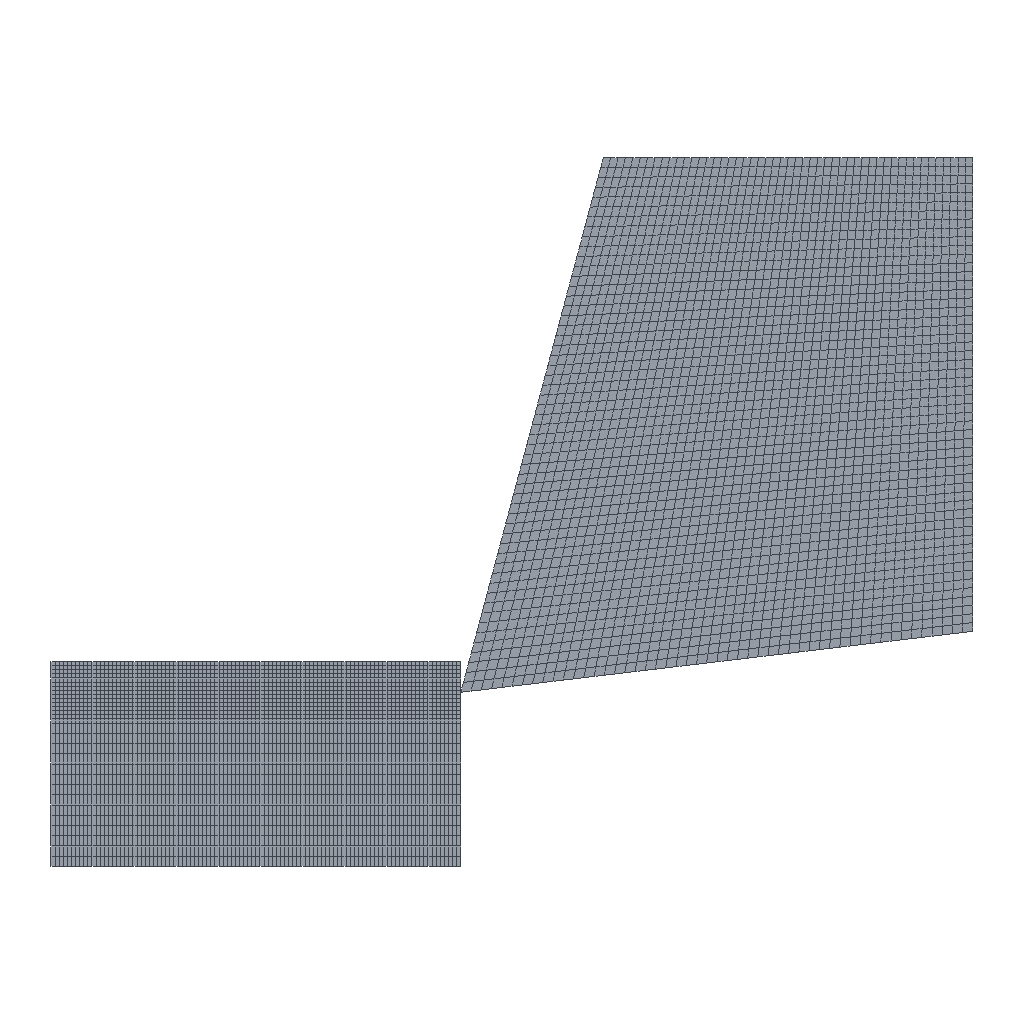Simulation study | abaqus
Set-up summary:
category,name,step,type,value,unit,region
solver,abaqus,,Abaqus/CAE 2024
units,mm-N-s-tonne (MPa),,inferred,E=960000 density=3.5e-09
analysis,Step-1,,dynamic temp-displacement,nlgeom=True; time_period=0.002
mesh,nodes,,,5836
mesh,elements,,,5600
element_type,CPE4RT,,,5600
material,DOMAND,,E,960000
material,DOMAND,,nu,0.2
material,DOMAND,,density,3.5e-09
material,DOMAND,,conductivity,1674.72
material,DOMAND,,specific_heat,5.16e+08
material,DOMAND,,cte,1.18e-06
material,DOMAND,,behaviors,conductivity; expansion; specific heat
material,TC4,,E,105000
material,TC4,,nu,0.33
material,TC4,,density,4.43e-09
material,TC4,,conductivity,5.44
material,TC4,,cte,9e-06
material,TC4,,behaviors,conductivity; damage initiation; damage evolution; expansion
section,TC4,,solid section,,,_PickedSet2
section,DOMAND,,solid section,,,_PickedSet2
load,Predefined,initial,initial condition temperature
bc,BC-1,initial,encastre,[dofs=ENCASTRE],,_PickedSet10
bc,BC-2,Step-1,velocity,"-1000 [dofs=rz,x,y n=3]",,_PickedSet11
contact,Int-1,Step-1,contact pair,interaction=INTPROP-1; friction=0.2; behavior=hard,,tool-1.Surf-tool / TC4-1_Set-all_CNS_
contact,Int-2,Step-1,general contact,interaction=IntProp-2
constraint,rigid body,,,1
Abaqus input file, long lists of numbers shortened:
*Heading
** Job name: deck Model name: Model-2-Copy
** Generated by: Abaqus/CAE 2024
*Preprint, echo=NO, model=NO, history=NO, contact=NO
**
** PARTS
**
*Part, name=TC4
*Node
      1,           2., -0.3
      2,           0., -0.3
** (3028 more lines like these left out)
*Element, type=CPE4RT
   1,    1,    7,  358,  230
   2,    7,    8,  359,  358
** (2898 more lines like these left out)
*Nset, nset=_PickedSet2, internal, generate
    1,  3030,     1
*Elset, elset=_PickedSet2, internal, generate
    1,  2900,     1
*Nset, nset=Set-all
    1,    2,    5,    6,    7,    8,    9,   10,   11,   12,   13,   14,   15,   16,   17,   18
   19,   20,   21,   22,   23,   24,   25,   26,   27,   28,   29,   30,   31,   32,   33,   34
** (99 more lines like these left out)
** Section: TC4
*Solid Section, elset=_PickedSet2, material=TC4
,
*End Part
**
*Part, name=tool
*Node
      1,           0.,           0.
      2, 0.05, 0.005956
** (2803 more lines like these left out)
*Element, type=CPE4RT
   1,    1,    2,   53,   52
   2,    2,    3,   54,   53
** (2698 more lines like these left out)
*Node
   2806,          2.5,   2.61,           0.
*Nset, nset=tool-RefPt_, internal
2806,
*Nset, nset=_PickedSet2, internal, generate
    1,  2805,     1
*Elset, elset=_PickedSet2, internal, generate
    1,  2700,     1
*Elset, elset=_Surf-tool_S1, internal, generate
  1,  50,   1
*Elset, elset=_Surf-tool_S4, internal, generate
    1,  2651,    50
*Surface, type=ELEMENT, name=Surf-tool
_Surf-tool_S1, S1
_Surf-tool_S4, S4
** Section: Tool
*Solid Section, elset=_PickedSet2, material=DOMAND
,
*End Part
**
**
** ASSEMBLY
**
*Assembly, name=Assembly
**
*Instance, name=TC4-1, part=TC4
*End Instance
**
*Instance, name=tool-1, part=tool
          2.,        -0.15,           0.
*End Instance
**
*Nset, nset=Set-RP, instance=tool-1
 2806,
*Nset, nset=_PickedSet6, internal, instance=tool-1
 2806,
*Nset, nset=_PickedSet7, internal, instance=tool-1, generate
    1,  2805,     1
*Elset, elset=_PickedSet7, internal, instance=tool-1, generate
    1,  2700,     1
*Nset, nset=_PickedSet9, internal, instance=tool-1
 2806,
*Nset, nset=_PickedSet10, internal, instance=TC4-1
   1,   2,   3,   4,   6, 106, 107, 108, 109, 110, 111, 112, 113, 114, 115, 116
 117, 118, 119, 120, 121, 122, 123, 124, 125, 126, 127, 128, 129, 130, 131, 132
** (7 more lines like these left out)
*Elset, elset=_PickedSet10, internal, instance=TC4-1
    1,  100,  101,  200,  201,  300,  301,  400,  401,  500,  501,  600,  601,  700,  701,  800
  801,  900,  901, 1000, 1001, 1100, 1101, 1200, 1201, 1300, 1301, 1302, 1303, 1304, 1305, 1306
** (7 more lines like these left out)
*Nset, nset=_PickedSet11, internal, instance=tool-1
 2806,
*Nset, nset=_PickedSet12, internal, instance=TC4-1, generate
    1,  3030,     1
*Nset, nset=_PickedSet12, internal, instance=tool-1, generate
    1,  2805,     1
*Elset, elset=_PickedSet12, internal, instance=TC4-1, generate
    1,  2900,     1
*Elset, elset=_PickedSet12, internal, instance=tool-1, generate
    1,  2700,     1
*Elset, elset=__PickedSurf8_S1, internal, instance=tool-1, generate
  1,  50,   1
*Elset, elset=__PickedSurf8_S2, internal, instance=tool-1, generate
   50,  2700,    50
*Elset, elset=__PickedSurf8_S4, internal, instance=tool-1, generate
    1,  2651,    50
*Surface, type=ELEMENT, name=_PickedSurf8, internal
__PickedSurf8_S1, S1
__PickedSurf8_S2, S2
__PickedSurf8_S4, S4
*Surface, type=NODE, name=TC4-1_Set-all_CNS_, internal
TC4-1.Set-all, 1.
** Constraint: Constraint-2
*Rigid Body, ref node=_PickedSet6, elset=_PickedSet7
*End Assembly
**
** MATERIALS
**
*Material, name=DOMAND
*Conductivity
 1674.72,
*Density
 3.5e-09,
*Elastic
960000., 0.2
*Expansion
 1.18e-06,
*Specific Heat
 5.16e+08,
*Material, name=TC4
*Conductivity
  5.44, 20.
   6.7,100.
  8.79,200.
 10.47,300.
 12.56,400.
 14.24,500.
 15.49,600.
*Damage Initiation, criterion=JOHNSON COOK
 -0.09,  0.25,  -0.5, 0.014,  3.87, 1650.,   20.,    1.
*Damage Evolution, type=DISPLACEMENT
 0.02,
*Density
 4.43e-09,
*Elastic
105000., 0.33
*Expansion
 9e-06,20.
*Inelastic Heat Fraction
        0.95,
*Plastic, hardening=JOHNSON COOK
875., 793., 0.38, 0.71,1650.,  20.
*Rate Dependent, type=JOHNSON COOK
 0.01,1.
*Specific Heat
 6.78e+08,100.
 6.91e+08,200.
 7.03e+08,300.
 7.41e+08,400.
 7.54e+08,500.
 8.79e+08,600.
**
** INTERACTION PROPERTIES
**
*Surface Interaction, name=INTPROP-1
*Friction
 0.2,
*Surface Behavior, pressure-overclosure=HARD
*Surface Interaction, name=IntProp-2
**
** BOUNDARY CONDITIONS
**
** Name: BC-1 Type: Symmetry/Antisymmetry/Encastre
*Boundary
_PickedSet10, ENCASTRE
**
** PREDEFINED FIELDS
**
** Name: Predefined Field-1   Type: Temperature
*Initial Conditions, type=TEMPERATURE
_PickedSet12, 25.
** ----------------------------------------------------------------
**
** STEP: Step-1
**
*Step, name=Step-1, nlgeom=YES
*Dynamic Temperature-displacement, Explicit
, 0.002
*Bulk Viscosity
0.06, 1.2
** Mass Scaling: Semi-Automatic
**               Whole Model
*Fixed Mass Scaling, factor=1000.
**
** BOUNDARY CONDITIONS
**
** Name: BC-2 Type: Velocity/Angular velocity
*Boundary, type=VELOCITY
_PickedSet11, 1, 1, -1000.
_PickedSet11, 2, 2
_PickedSet11, 6, 6
**
** INTERACTIONS
**
** Interaction: Int-1
*Contact Pair, interaction=INTPROP-1, mechanical constraint=PENALTY, cpset=Int-1
tool-1.Surf-tool, TC4-1_Set-all_CNS_
** Interaction: Int-2
*Contact, op=NEW
*Contact Inclusions, ALL EXTERIOR
*Contact Property Assignment
 ,  , IntProp-2
**
** OUTPUT REQUESTS
**
*Restart, write, number interval=1, time marks=NO
**
** FIELD OUTPUT: F-Output-1
**
*Output, field, number interval=500
*Node Output
NT, RF
*Element Output, directions=YES
CFAILURE, DAMAGESHR, DMICRT, E, EVF, S, SDEG, STATUS, TEMP
*Contact Output
CSDMG, CSTRESS
*Output, history, frequency=0
*End Step
Results summary:
result,odb.job_status,,,JOB_STATUS_UNKNOWN,"consistent, unstated (Abaqus has no unit system)"
result,steps[0].procedure,Step-1,,"*DYNAMIC TEMPERATURE-DISPLACEMENT, EXPLICT","consistent, unstated (Abaqus has no unit system)"
result,steps[0].time_period,Step-1,,0.002,"consistent, unstated (Abaqus has no unit system)"
result,steps[0].n_frames,Step-1,,229,"consistent, unstated (Abaqus has no unit system)"
result,steps[0].last_frame.id,Step-1,,10414,"consistent, unstated (Abaqus has no unit system)"
result,steps[0].last_frame.value,Step-1,,0.000912,"consistent, unstated (Abaqus has no unit system)"
result,steps[0].last_frame.description,Step-1,,Increment     10414: Step Time =   9.1205E-04,"consistent, unstated (Abaqus has no unit system)"
result,steps[0].completed,Step-1,,False,"consistent, unstated (Abaqus has no unit system)"
result,steps[0].max_U_magnitude,Step-1,,5.856,"consistent, unstated (Abaqus has no unit system)"
result,steps[0].max_S_mises,Step-1,,1147.01,"consistent, unstated (Abaqus has no unit system)"
result,steps[0].RF_sum[1],Step-1,,132.127,"consistent, unstated (Abaqus has no unit system)"
result,steps[0].RF_sum[2],Step-1,,46.478,"consistent, unstated (Abaqus has no unit system)"
result,steps[0].diagnostic.n_increments,Step-1,,229,"consistent, unstated (Abaqus has no unit system)"